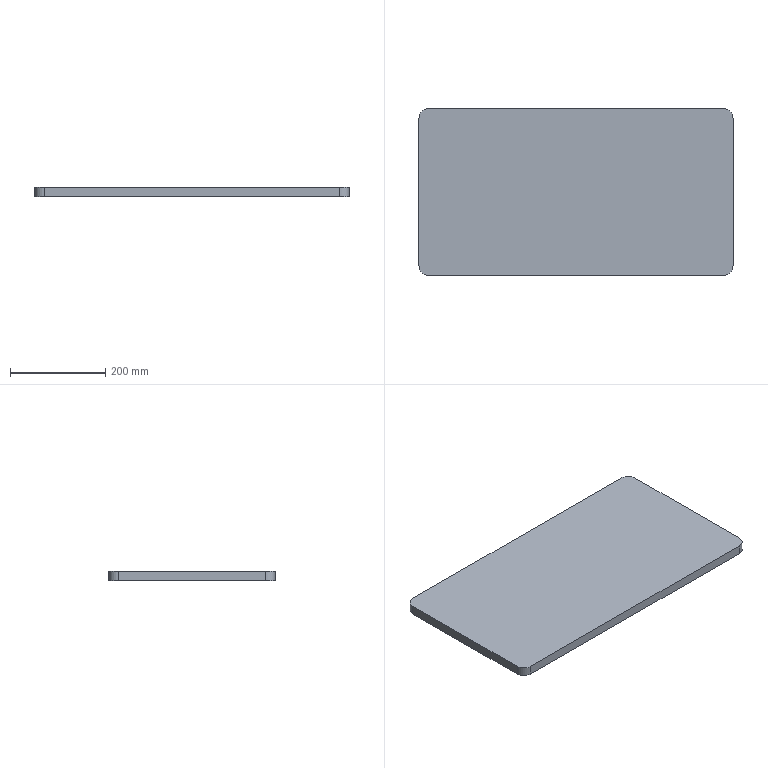Part | STEP file | 09-34 front table plate | 1 solid | 10 faces | box 660 x 350 x 20 mm | volume 4613133 mm3 | plane 6 | cylinder 4 | commonest cylinder face diameters 40 x4
STEP:
#1=CARTESIAN_POINT('',(330.,-155.,0.));
#2=VERTEX_POINT('',#1);
#3=CARTESIAN_POINT('',(330.,155.,0.));
#4=VERTEX_POINT('',#3);
#5=CARTESIAN_POINT('',(330.,175.,0.));
#6=DIRECTION('',(0.,1.,0.));
#7=VECTOR('',#6,1000.);
#8=LINE('',#5,#7);
#9=EDGE_CURVE('',#2,#4,#8,.T.);
#10=ORIENTED_EDGE('',*,*,#9,.T.);
#11=CARTESIAN_POINT('',(330.,155.,20.));
#12=VERTEX_POINT('',#11);
#13=CARTESIAN_POINT('',(330.,155.,20.));
#14=DIRECTION('',(0.,0.,1.));
#15=VECTOR('',#14,1000.);
#16=LINE('',#13,#15);
#17=EDGE_CURVE('',#4,#12,#16,.T.);
#18=ORIENTED_EDGE('',*,*,#17,.T.);
#19=CARTESIAN_POINT('',(330.,-155.,20.));
#20=VERTEX_POINT('',#19);
#21=CARTESIAN_POINT('',(330.,175.,20.));
#22=DIRECTION('',(0.,1.,0.));
#23=VECTOR('',#22,1000.);
#24=LINE('',#21,#23);
#25=EDGE_CURVE('',#20,#12,#24,.T.);
#26=ORIENTED_EDGE('',*,*,#25,.F.);
#27=CARTESIAN_POINT('',(330.,-155.,20.));
#28=DIRECTION('',(0.,0.,-1.));
#29=VECTOR('',#28,1000.);
#30=LINE('',#27,#29);
#31=EDGE_CURVE('',#20,#2,#30,.T.);
#32=ORIENTED_EDGE('',*,*,#31,.T.);
#33=EDGE_LOOP('',(#10,#18,#26,#32));
#34=FACE_OUTER_BOUND('',#33,.T.);
#35=CARTESIAN_POINT('',(330.,175.,20.));
#36=DIRECTION('',(-1.,0.,0.));
#37=DIRECTION('',(0.,-1.,0.));
#38=AXIS2_PLACEMENT_3D('',#35,#36,#37);
#39=PLANE('',#38);
#40=ADVANCED_FACE('',(#34),#39,.F.);
#41=CARTESIAN_POINT('',(310.,175.,0.));
#42=VERTEX_POINT('',#41);
#43=CARTESIAN_POINT('',(-310.,175.,0.));
#44=VERTEX_POINT('',#43);
#45=CARTESIAN_POINT('',(-330.,175.,0.));
#46=DIRECTION('',(-1.,0.,0.));
#47=VECTOR('',#46,1000.);
#48=LINE('',#45,#47);
#49=EDGE_CURVE('',#42,#44,#48,.T.);
#50=ORIENTED_EDGE('',*,*,#49,.T.);
#51=CARTESIAN_POINT('',(-310.,175.,20.));
#52=VERTEX_POINT('',#51);
#53=CARTESIAN_POINT('',(-310.,175.,20.));
#54=DIRECTION('',(0.,0.,1.));
#55=VECTOR('',#54,1000.);
#56=LINE('',#53,#55);
#57=EDGE_CURVE('',#44,#52,#56,.T.);
#58=ORIENTED_EDGE('',*,*,#57,.T.);
#59=CARTESIAN_POINT('',(310.,175.,20.));
#60=VERTEX_POINT('',#59);
#61=CARTESIAN_POINT('',(-330.,175.,20.));
#62=DIRECTION('',(-1.,0.,0.));
#63=VECTOR('',#62,1000.);
#64=LINE('',#61,#63);
#65=EDGE_CURVE('',#60,#52,#64,.T.);
#66=ORIENTED_EDGE('',*,*,#65,.F.);
#67=CARTESIAN_POINT('',(310.,175.,20.));
#68=DIRECTION('',(0.,0.,-1.));
#69=VECTOR('',#68,1000.);
#70=LINE('',#67,#69);
#71=EDGE_CURVE('',#60,#42,#70,.T.);
#72=ORIENTED_EDGE('',*,*,#71,.T.);
#73=EDGE_LOOP('',(#50,#58,#66,#72));
#74=FACE_OUTER_BOUND('',#73,.T.);
#75=CARTESIAN_POINT('',(-330.,175.,20.));
#76=DIRECTION('',(0.,-1.,0.));
#77=DIRECTION('',(0.,0.,-1.));
#78=AXIS2_PLACEMENT_3D('',#75,#76,#77);
#79=PLANE('',#78);
#80=ADVANCED_FACE('',(#74),#79,.F.);
#81=CARTESIAN_POINT('',(-330.,155.,20.));
#82=VERTEX_POINT('',#81);
#83=CARTESIAN_POINT('',(-330.,-155.,20.));
#84=VERTEX_POINT('',#83);
#85=CARTESIAN_POINT('',(-330.,175.,20.));
#86=DIRECTION('',(0.,-1.,0.));
#87=VECTOR('',#86,1000.);
#88=LINE('',#85,#87);
#89=EDGE_CURVE('',#82,#84,#88,.T.);
#90=ORIENTED_EDGE('',*,*,#89,.F.);
#91=CARTESIAN_POINT('',(-330.,155.,0.));
#92=VERTEX_POINT('',#91);
#93=CARTESIAN_POINT('',(-330.,155.,20.));
#94=DIRECTION('',(0.,0.,-1.));
#95=VECTOR('',#94,1000.);
#96=LINE('',#93,#95);
#97=EDGE_CURVE('',#82,#92,#96,.T.);
#98=ORIENTED_EDGE('',*,*,#97,.T.);
#99=CARTESIAN_POINT('',(-330.,-155.,0.));
#100=VERTEX_POINT('',#99);
#101=CARTESIAN_POINT('',(-330.,175.,0.));
#102=DIRECTION('',(0.,-1.,0.));
#103=VECTOR('',#102,1000.);
#104=LINE('',#101,#103);
#105=EDGE_CURVE('',#92,#100,#104,.T.);
#106=ORIENTED_EDGE('',*,*,#105,.T.);
#107=CARTESIAN_POINT('',(-330.,-155.,20.));
#108=DIRECTION('',(0.,0.,1.));
#109=VECTOR('',#108,1000.);
#110=LINE('',#107,#109);
#111=EDGE_CURVE('',#100,#84,#110,.T.);
#112=ORIENTED_EDGE('',*,*,#111,.T.);
#113=EDGE_LOOP('',(#90,#98,#106,#112));
#114=FACE_OUTER_BOUND('',#113,.T.);
#115=CARTESIAN_POINT('',(-330.,175.,20.));
#116=DIRECTION('',(1.,0.,0.));
#117=DIRECTION('',(0.,1.,0.));
#118=AXIS2_PLACEMENT_3D('',#115,#116,#117);
#119=PLANE('',#118);
#120=ADVANCED_FACE('',(#114),#119,.F.);
#121=CARTESIAN_POINT('',(-310.,-175.,0.));
#122=VERTEX_POINT('',#121);
#123=CARTESIAN_POINT('',(310.,-175.,0.));
#124=VERTEX_POINT('',#123);
#125=CARTESIAN_POINT('',(-330.,-175.,0.));
#126=DIRECTION('',(1.,0.,0.));
#127=VECTOR('',#126,1000.);
#128=LINE('',#125,#127);
#129=EDGE_CURVE('',#122,#124,#128,.T.);
#130=ORIENTED_EDGE('',*,*,#129,.T.);
#131=CARTESIAN_POINT('',(310.,-175.,20.));
#132=VERTEX_POINT('',#131);
#133=CARTESIAN_POINT('',(310.,-175.,20.));
#134=DIRECTION('',(0.,0.,1.));
#135=VECTOR('',#134,1000.);
#136=LINE('',#133,#135);
#137=EDGE_CURVE('',#124,#132,#136,.T.);
#138=ORIENTED_EDGE('',*,*,#137,.T.);
#139=CARTESIAN_POINT('',(-310.,-175.,20.));
#140=VERTEX_POINT('',#139);
#141=CARTESIAN_POINT('',(-330.,-175.,20.));
#142=DIRECTION('',(1.,0.,0.));
#143=VECTOR('',#142,1000.);
#144=LINE('',#141,#143);
#145=EDGE_CURVE('',#140,#132,#144,.T.);
#146=ORIENTED_EDGE('',*,*,#145,.F.);
#147=CARTESIAN_POINT('',(-310.,-175.,20.));
#148=DIRECTION('',(0.,0.,-1.));
#149=VECTOR('',#148,1000.);
#150=LINE('',#147,#149);
#151=EDGE_CURVE('',#140,#122,#150,.T.);
#152=ORIENTED_EDGE('',*,*,#151,.T.);
#153=EDGE_LOOP('',(#130,#138,#146,#152));
#154=FACE_OUTER_BOUND('',#153,.T.);
#155=CARTESIAN_POINT('',(-330.,-175.,20.));
#156=DIRECTION('',(0.,1.,0.));
#157=DIRECTION('',(0.,0.,1.));
#158=AXIS2_PLACEMENT_3D('',#155,#156,#157);
#159=PLANE('',#158);
#160=ADVANCED_FACE('',(#154),#159,.F.);
#161=ORIENTED_EDGE('',*,*,#65,.T.);
#162=CARTESIAN_POINT('',(-310.,155.,20.));
#163=DIRECTION('',(0.,0.,1.));
#164=DIRECTION('',(1.,0.,0.));
#165=AXIS2_PLACEMENT_3D('',#162,#163,#164);
#166=CIRCLE('',#165,20.);
#167=EDGE_CURVE('',#52,#82,#166,.T.);
#168=ORIENTED_EDGE('',*,*,#167,.T.);
#169=ORIENTED_EDGE('',*,*,#89,.T.);
#170=CARTESIAN_POINT('',(-310.,-155.,20.));
#171=DIRECTION('',(0.,0.,1.));
#172=DIRECTION('',(1.,0.,0.));
#173=AXIS2_PLACEMENT_3D('',#170,#171,#172);
#174=CIRCLE('',#173,20.);
#175=EDGE_CURVE('',#84,#140,#174,.T.);
#176=ORIENTED_EDGE('',*,*,#175,.T.);
#177=ORIENTED_EDGE('',*,*,#145,.T.);
#178=CARTESIAN_POINT('',(310.,-155.,20.));
#179=DIRECTION('',(0.,0.,1.));
#180=DIRECTION('',(1.,0.,0.));
#181=AXIS2_PLACEMENT_3D('',#178,#179,#180);
#182=CIRCLE('',#181,20.);
#183=EDGE_CURVE('',#132,#20,#182,.T.);
#184=ORIENTED_EDGE('',*,*,#183,.T.);
#185=ORIENTED_EDGE('',*,*,#25,.T.);
#186=CARTESIAN_POINT('',(310.,155.,20.));
#187=DIRECTION('',(0.,0.,1.));
#188=DIRECTION('',(1.,0.,0.));
#189=AXIS2_PLACEMENT_3D('',#186,#187,#188);
#190=CIRCLE('',#189,20.);
#191=EDGE_CURVE('',#12,#60,#190,.T.);
#192=ORIENTED_EDGE('',*,*,#191,.T.);
#193=EDGE_LOOP('',(#161,#168,#169,#176,#177,#184,#185,#192));
#194=FACE_OUTER_BOUND('',#193,.T.);
#195=CARTESIAN_POINT('',(330.,-175.,20.));
#196=DIRECTION('',(0.,0.,1.));
#197=DIRECTION('',(1.,0.,0.));
#198=AXIS2_PLACEMENT_3D('',#195,#196,#197);
#199=PLANE('',#198);
#200=ADVANCED_FACE('',(#194),#199,.T.);
#201=ORIENTED_EDGE('',*,*,#105,.F.);
#202=CARTESIAN_POINT('',(-310.,155.,0.));
#203=DIRECTION('',(0.,0.,-1.));
#204=DIRECTION('',(1.,0.,0.));
#205=AXIS2_PLACEMENT_3D('',#202,#203,#204);
#206=CIRCLE('',#205,20.);
#207=EDGE_CURVE('',#92,#44,#206,.T.);
#208=ORIENTED_EDGE('',*,*,#207,.T.);
#209=ORIENTED_EDGE('',*,*,#49,.F.);
#210=CARTESIAN_POINT('',(310.,155.,0.));
#211=DIRECTION('',(0.,0.,-1.));
#212=DIRECTION('',(1.,0.,0.));
#213=AXIS2_PLACEMENT_3D('',#210,#211,#212);
#214=CIRCLE('',#213,20.);
#215=EDGE_CURVE('',#42,#4,#214,.T.);
#216=ORIENTED_EDGE('',*,*,#215,.T.);
#217=ORIENTED_EDGE('',*,*,#9,.F.);
#218=CARTESIAN_POINT('',(310.,-155.,0.));
#219=DIRECTION('',(0.,0.,-1.));
#220=DIRECTION('',(1.,0.,0.));
#221=AXIS2_PLACEMENT_3D('',#218,#219,#220);
#222=CIRCLE('',#221,20.);
#223=EDGE_CURVE('',#2,#124,#222,.T.);
#224=ORIENTED_EDGE('',*,*,#223,.T.);
#225=ORIENTED_EDGE('',*,*,#129,.F.);
#226=CARTESIAN_POINT('',(-310.,-155.,0.));
#227=DIRECTION('',(0.,0.,-1.));
#228=DIRECTION('',(1.,0.,0.));
#229=AXIS2_PLACEMENT_3D('',#226,#227,#228);
#230=CIRCLE('',#229,20.);
#231=EDGE_CURVE('',#122,#100,#230,.T.);
#232=ORIENTED_EDGE('',*,*,#231,.T.);
#233=EDGE_LOOP('',(#201,#208,#209,#216,#217,#224,#225,#232));
#234=FACE_OUTER_BOUND('',#233,.T.);
#235=CARTESIAN_POINT('',(330.,-175.,0.));
#236=DIRECTION('',(0.,0.,1.));
#237=DIRECTION('',(1.,0.,0.));
#238=AXIS2_PLACEMENT_3D('',#235,#236,#237);
#239=PLANE('',#238);
#240=ADVANCED_FACE('',(#234),#239,.F.);
#241=ORIENTED_EDGE('',*,*,#167,.F.);
#242=ORIENTED_EDGE('',*,*,#57,.F.);
#243=ORIENTED_EDGE('',*,*,#207,.F.);
#244=ORIENTED_EDGE('',*,*,#97,.F.);
#245=EDGE_LOOP('',(#241,#242,#243,#244));
#246=FACE_OUTER_BOUND('',#245,.T.);
#247=CARTESIAN_POINT('',(-310.,155.,20.));
#248=DIRECTION('',(0.,0.,-1.));
#249=DIRECTION('',(-1.,0.,0.));
#250=AXIS2_PLACEMENT_3D('',#247,#248,#249);
#251=CYLINDRICAL_SURFACE('',#250,20.);
#252=ADVANCED_FACE('',(#246),#251,.T.);
#253=ORIENTED_EDGE('',*,*,#191,.F.);
#254=ORIENTED_EDGE('',*,*,#17,.F.);
#255=ORIENTED_EDGE('',*,*,#215,.F.);
#256=ORIENTED_EDGE('',*,*,#71,.F.);
#257=EDGE_LOOP('',(#253,#254,#255,#256));
#258=FACE_OUTER_BOUND('',#257,.T.);
#259=CARTESIAN_POINT('',(310.,155.,20.));
#260=DIRECTION('',(0.,0.,-1.));
#261=DIRECTION('',(-1.,0.,0.));
#262=AXIS2_PLACEMENT_3D('',#259,#260,#261);
#263=CYLINDRICAL_SURFACE('',#262,20.);
#264=ADVANCED_FACE('',(#258),#263,.T.);
#265=ORIENTED_EDGE('',*,*,#183,.F.);
#266=ORIENTED_EDGE('',*,*,#137,.F.);
#267=ORIENTED_EDGE('',*,*,#223,.F.);
#268=ORIENTED_EDGE('',*,*,#31,.F.);
#269=EDGE_LOOP('',(#265,#266,#267,#268));
#270=FACE_OUTER_BOUND('',#269,.T.);
#271=CARTESIAN_POINT('',(310.,-155.,20.));
#272=DIRECTION('',(0.,0.,-1.));
#273=DIRECTION('',(-1.,0.,0.));
#274=AXIS2_PLACEMENT_3D('',#271,#272,#273);
#275=CYLINDRICAL_SURFACE('',#274,20.);
#276=ADVANCED_FACE('',(#270),#275,.T.);
#277=ORIENTED_EDGE('',*,*,#175,.F.);
#278=ORIENTED_EDGE('',*,*,#111,.F.);
#279=ORIENTED_EDGE('',*,*,#231,.F.);
#280=ORIENTED_EDGE('',*,*,#151,.F.);
#281=EDGE_LOOP('',(#277,#278,#279,#280));
#282=FACE_OUTER_BOUND('',#281,.T.);
#283=CARTESIAN_POINT('',(-310.,-155.,20.));
#284=DIRECTION('',(0.,0.,-1.));
#285=DIRECTION('',(-1.,0.,0.));
#286=AXIS2_PLACEMENT_3D('',#283,#284,#285);
#287=CYLINDRICAL_SURFACE('',#286,20.);
#288=ADVANCED_FACE('',(#282),#287,.T.);
#289=CLOSED_SHELL('',(#40,#80,#120,#160,#200,#240,#252,#264,#276,#288));
#290=MANIFOLD_SOLID_BREP('',#289);
#291=CARTESIAN_POINT('',(0.,0.,0.));
#292=DIRECTION('',(0.,0.,1.));
#293=DIRECTION('',(1.,0.,0.));
#294=AXIS2_PLACEMENT_3D('',#291,#292,#293);
#295=(LENGTH_UNIT()NAMED_UNIT(*)SI_UNIT(.MILLI.,.METRE.));
#296=UNCERTAINTY_MEASURE_WITH_UNIT(LENGTH_MEASURE(0.00001),#295,'','');
#297=(NAMED_UNIT(*)PLANE_ANGLE_UNIT()SI_UNIT($,.RADIAN.));
#298=(NAMED_UNIT(*)SI_UNIT($,.STERADIAN.)SOLID_ANGLE_UNIT());
#299=(GEOMETRIC_REPRESENTATION_CONTEXT(3)GLOBAL_UNCERTAINTY_ASSIGNED_CONTEXT((#296))GLOBAL_UNIT_ASSIGNED_CONTEXT((#295,#297,#298))REPRESENTATION_CONTEXT('',''));
#300=ADVANCED_BREP_SHAPE_REPRESENTATION('',(#290,#294),#299);